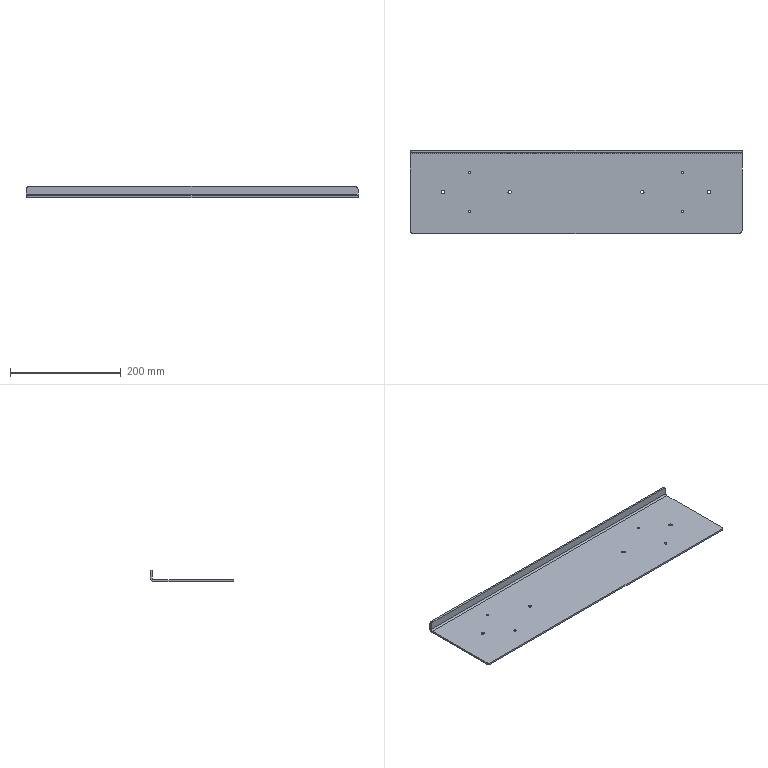Part | STEP file | J452-EBZ05-25-08-Part-1 | 1 solid | 30 faces | box 600 x 150 x 20 mm | volume 296591 mm3 | cylinder 22 | plane 8 | commonest cylinder face diameters 4 x8 5.8 x8 10 x4 6 x1 12 x1